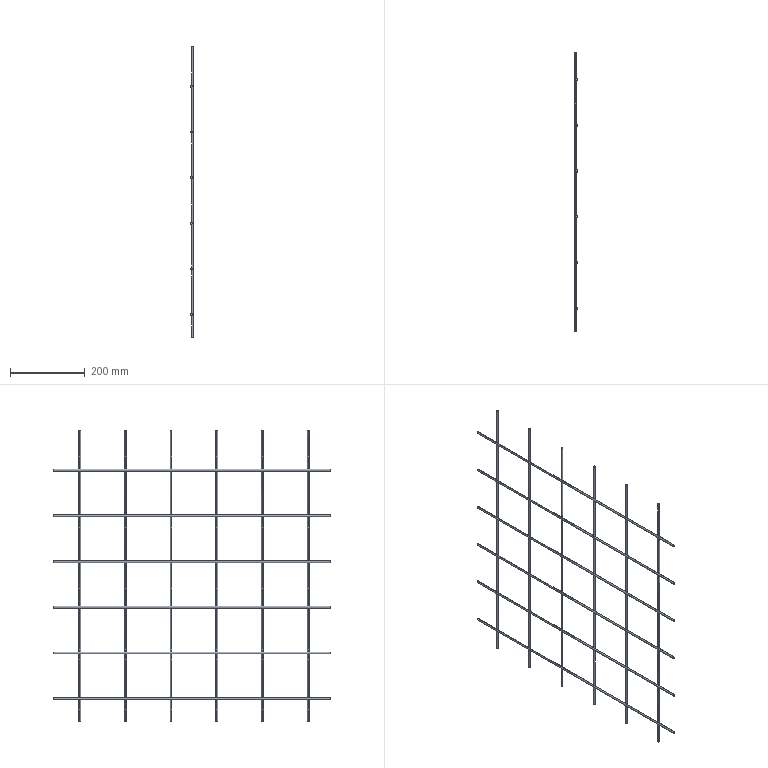Part | SolidWorks | features BaseBody 1, ICE 1, MirrorPattern 1 | 1 solid | 48 faces | box 8 x 742 x 777 mm | volume 178056 mm3 | cylinder 24 | plane 24 | commonest cylinder face diameters 5 x24